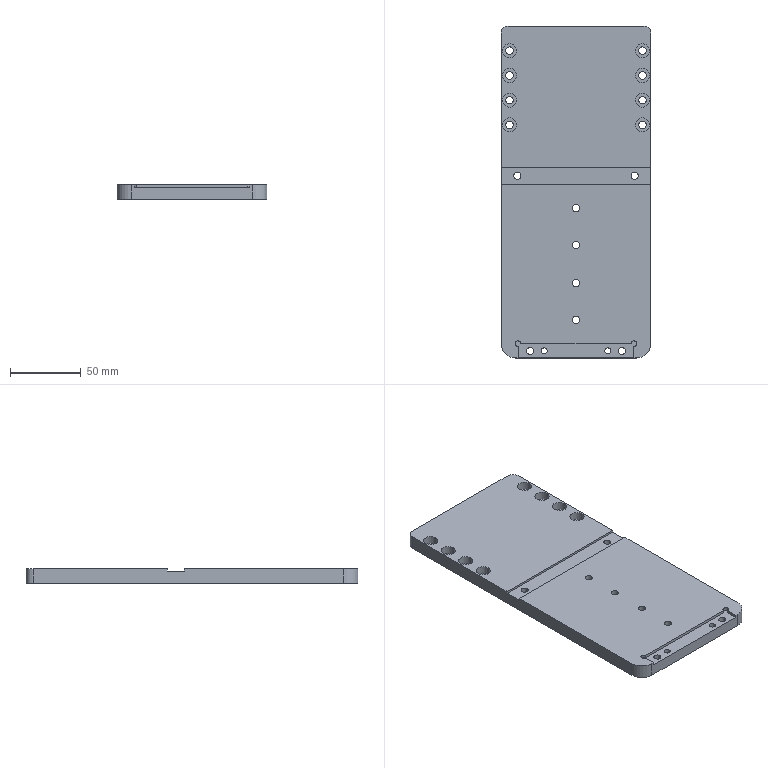Part | SolidWorks | features HoleWzd 7, ICE 5, Fillet 2, Extrusion 1, LPattern 1, MirrorPattern 1, MoveFace 1 | 1 solid | 87 faces | box 106 x 235 x 10 mm | volume 238418 mm3 | cylinder 63 | plane 24 | commonest cylinder face diameters 10 x18 5 x16 5.4 x16 4.3 x4 8 x4 4 x3